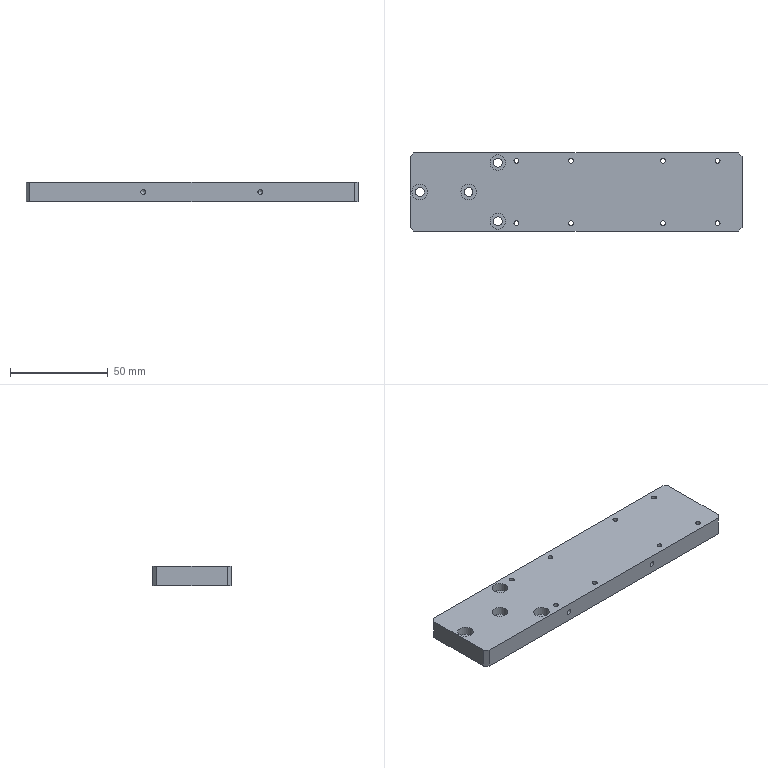CAM job | NX | 3-axis milling, drilling | part box 170 x 40 x 10 mm | stock box 175 x 45 x 12 mm
Tools:
number,name,description,diameter,corner_radius,flute_length,length,flutes
4,D4,平底铣刀-粗,4.0,0.0,25.0,75.0,2
9,D10,平底铣刀-粗,10.0,0.0,35.0,75.0,2
10,D10-J,平底铣刀-精,10.0,0.0,35.0,75.0,2
1,D80R0.8飞刀,圆鼻刀-粗,80.0,0.8,50.0,75.0,2
2,D6倒角刀,倒角刀,6.0,0.0,3.0,25.0,2
20,M3X0.5,丝锥,2.5,0.0,35.0,50.0,2
12,ZT2.5,钻头,2.5,0.0,35.0,50.0,2
11,ZT4.5,钻头,4.5,0.0,35.0,50.0,2
Operations:
program,operation,operation_type,tool,method,geometry_group,spindle_rpm,surface_speed,feed_per_tooth,feed_cut,feed_plunge,cut_length_mm,path_length_mm,cut_time_min,machine_time_min
B,FACEMILL_AUTOROUGH_1PASS_COPY,FaceMilling,D80R0.8飞刀,LAYERROUGH-DEPTHK-STEPG,W-B,4500.0,890.615,0.3333,3000.0,100.0,1112.0,1978.65,0.3707,0.4573
B,FACEMILL_AUTOFINISH_1PASS_COPY,FaceMilling,D80R0.8飞刀,SIDEFINISH-DEPTHK-STEPG,W-B,4500.0,890.615,0.1111,1000.0,100.0,278.0,314.0,0.278,0.2816
B,DRILLCHAMFER_2,Operation,D6倒角刀,METHOD,W-B,8000.0,150.796,0.0625,1000.0,0.0,38.0,361.017,0.038,0.0703
B,DRILLCHAMFER_3,Operation,D6倒角刀,METHOD,W-B,8000.0,150.796,0.0625,1000.0,0.0,22.2,170.153,0.0222,0.037
B,C0.3_CLOSEDCONTOURCHAMFER6X45L_COPY,PlanarMilling,D6倒角刀,WALLCLIMB_CHAMFER-DEPTH0-STEPG,W-B,7000.0,131.0,0.1071,1500.0,100.0,432.842,468.842,0.2886,0.2922
A,TOPFACE,FaceMilling,D80R0.8飞刀,SIDEFINISH-DEPTHK-STEPG,W-A,4000.0,1005.31,0.125,1000.0,100.0,264.0,300.0,0.264,0.2676
A,PROFILE_ROUGH_2,VolumeBased25DMillingOperation,D10,METHOD,W-A,8000.0,251.327,0.3125,5000.0,80.0,6711.878,6760.478,1.342,1.347
A,SPOT-DEPTH0.8,Operation,D6倒角刀,NONE,W-A,8000.0,150.796,0.0312,500.0,90.0,21.6,387.2,0.0432,0.0798
A,THROUGHHOLE-M3TAPDRILL,Operation,ZT2.5,NONE,W-A,3000.0,23.562,0.05,300.0,90.0,134.009,538.13,0.4467,0.4871
A,COUNTERBOREHOLE-DRILL0SEG,Operation,ZT4.5,NONE,W-A,2800.0,39.584,0.0179,100.0,90.0,57.408,234.089,0.5741,0.5917
A,HOLEROUGH_D4_1,CylinderMilling,D4,NONE,W-A,8000.0,100.531,0.075,1200.0,100.0,851.827,1103.64,0.7099,0.735
A,HOLEFINISH_D4_1,CylinderMilling,D4,FINISHSTEPDEPTHOFF,W-A,8000.0,100.531,0.0312,500.0,100.0,128.184,379.998,0.2564,0.2816
A,SELECTBODYONLY,SurfaceContour,D6倒角刀,METHOD,W-A,8000.0,150.796,0.1875,3000.0,100.0,432.615,468.416,0.1442,0.1478
A,DRILLCHAMFER_1,Operation,D6倒角刀,METHOD,W-A,8000.0,150.796,0.0312,500.0,0.0,38.0,361.017,0.076,0.1083
A,MILLCHAMFER_1,PlanarMilling,D6倒角刀,NONE,W-A,8000.0,150.796,0.0312,500.0,100.0,135.871,367.771,0.2717,0.2949
A,THROUGHHOLE-TAPM3,Operation,M3X0.5,METHOD,W-A,800.0,6.283,0.0003,0.5,90.0,112.0,494.113,224.0,224.038
A,PROFILE_SEMI_2,VolumeBased25DMillingOperation,D10-J,METHOD,W-A,8000.0,251.327,0.0625,1000.0,100.0,451.688,510.888,0.4517,0.4576